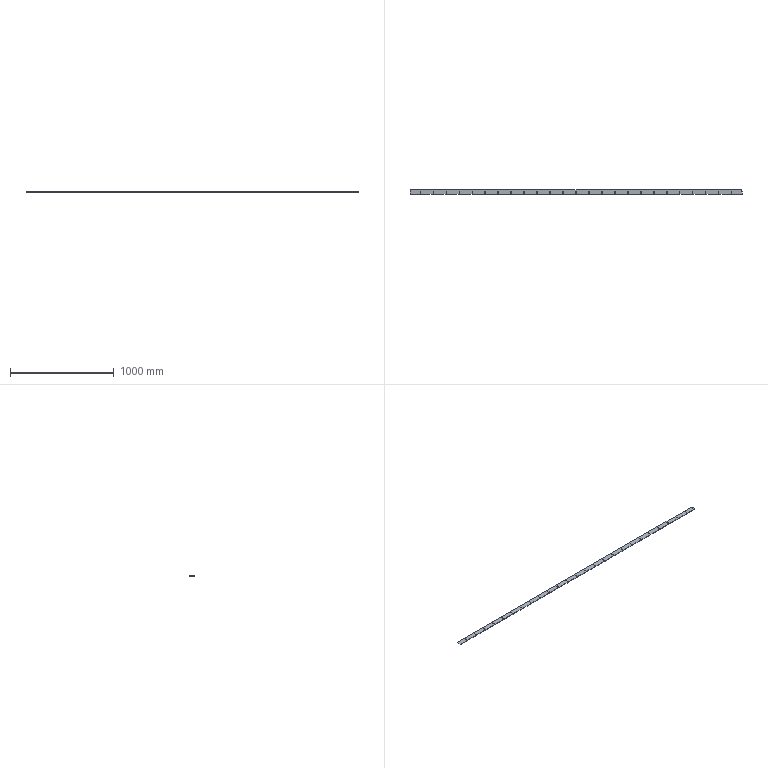Part | SolidWorks | features Fillet 1, FlatPattern 1, SMBaseFlange 1, SheetMetal 1 | 1 solid | 114 faces | box 3200 x 45 x 4.5 mm | volume 632235 mm3 | plane 110 | cylinder 4 | commonest cylinder face diameters 2 x4